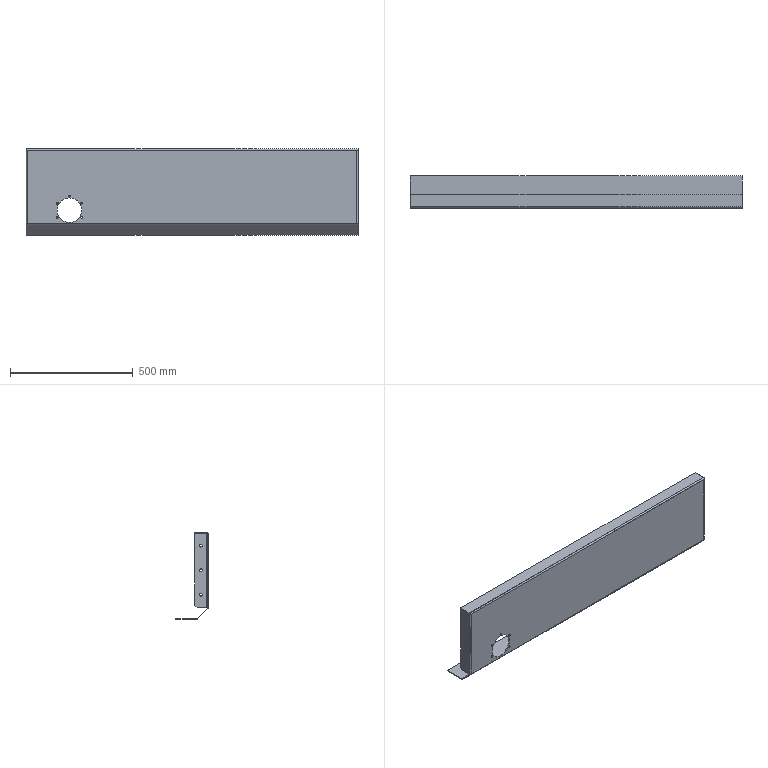Part | STEP file | VD-SYL0380DJ1006_1_3-1_VD-SYL03 | 1 solid | 78 faces | box 1354 x 132 x 353 mm | volume 2119091 mm3 | plane 44 | cylinder 34 | commonest cylinder face diameters 11 x12 8 x10 6 x5 12 x5 100 x2